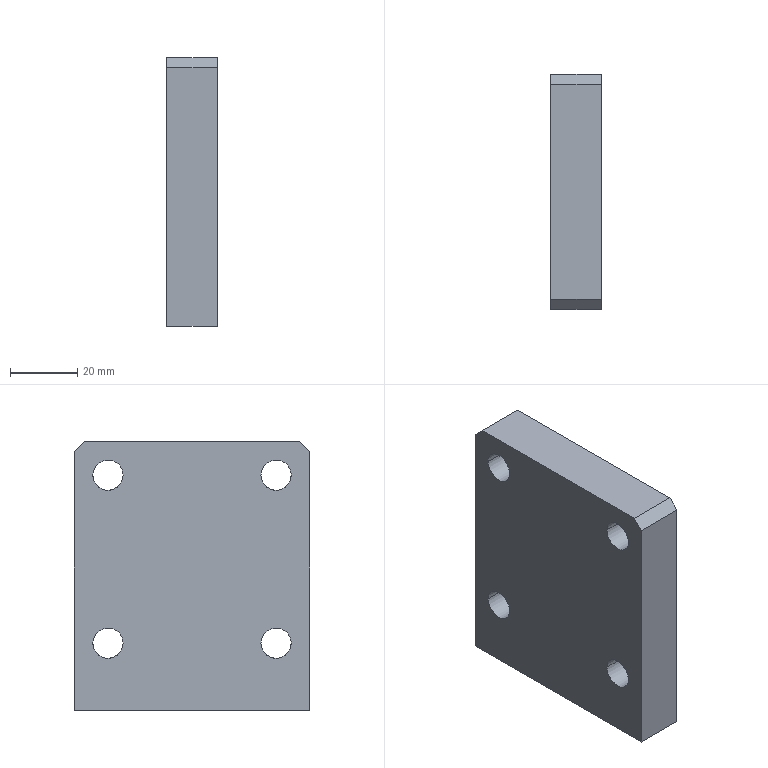Part | STEP file | Positioning_id1926_x_t | 1 solid | 16 faces | box 15 x 70 x 80 mm | volume 80048 mm3 | cylinder 8 | plane 8 | commonest cylinder face diameters 9 x8